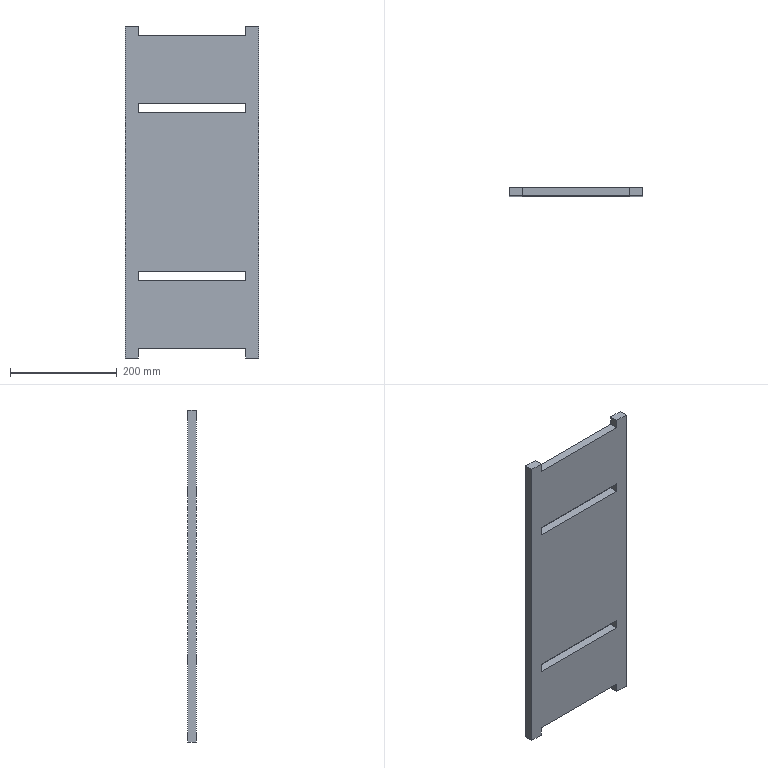Part | SolidWorks | features Extrusion 1 | 1 solid | 22 faces | box 250 x 16 x 623 mm | volume 2273312 mm3 | plane 22
STEP:
#1=CARTESIAN_POINT('',(-100.5,0.,165.5));
#2=VERTEX_POINT('',#1);
#3=CARTESIAN_POINT('',(100.5,0.,165.5));
#4=VERTEX_POINT('',#3);
#5=CARTESIAN_POINT('',(0.,0.,165.5));
#6=DIRECTION('',(1.,0.,0.));
#7=VECTOR('',#6,1000.);
#8=LINE('',#5,#7);
#9=EDGE_CURVE('',#2,#4,#8,.T.);
#10=ORIENTED_EDGE('',*,*,#9,.F.);
#11=CARTESIAN_POINT('',(-100.5,16.,165.5));
#12=VERTEX_POINT('',#11);
#13=CARTESIAN_POINT('',(-100.5,16.,165.5));
#14=DIRECTION('',(0.,-1.,0.));
#15=VECTOR('',#14,1000.);
#16=LINE('',#13,#15);
#17=EDGE_CURVE('',#12,#2,#16,.T.);
#18=ORIENTED_EDGE('',*,*,#17,.F.);
#19=CARTESIAN_POINT('',(100.5,16.,165.5));
#20=VERTEX_POINT('',#19);
#21=CARTESIAN_POINT('',(0.,16.,165.5));
#22=DIRECTION('',(1.,0.,0.));
#23=VECTOR('',#22,1000.);
#24=LINE('',#21,#23);
#25=EDGE_CURVE('',#12,#20,#24,.T.);
#26=ORIENTED_EDGE('',*,*,#25,.T.);
#27=CARTESIAN_POINT('',(100.5,16.,165.5));
#28=DIRECTION('',(0.,-1.,0.));
#29=VECTOR('',#28,1000.);
#30=LINE('',#27,#29);
#31=EDGE_CURVE('',#20,#4,#30,.T.);
#32=ORIENTED_EDGE('',*,*,#31,.T.);
#33=EDGE_LOOP('',(#10,#18,#26,#32));
#34=FACE_OUTER_BOUND('',#33,.T.);
#35=CARTESIAN_POINT('',(0.,16.,165.5));
#36=DIRECTION('',(0.,0.,-1.));
#37=DIRECTION('',(-1.,0.,0.));
#38=AXIS2_PLACEMENT_3D('',#35,#36,#37);
#39=PLANE('',#38);
#40=ADVANCED_FACE('',(#34),#39,.T.);
#41=CARTESIAN_POINT('',(-100.5,0.,148.5));
#42=VERTEX_POINT('',#41);
#43=CARTESIAN_POINT('',(-100.5,0.,0.));
#44=DIRECTION('',(0.,0.,-1.));
#45=VECTOR('',#44,1000.);
#46=LINE('',#43,#45);
#47=EDGE_CURVE('',#2,#42,#46,.T.);
#48=ORIENTED_EDGE('',*,*,#47,.T.);
#49=CARTESIAN_POINT('',(-100.5,16.,148.5));
#50=VERTEX_POINT('',#49);
#51=CARTESIAN_POINT('',(-100.5,16.,148.5));
#52=DIRECTION('',(0.,-1.,0.));
#53=VECTOR('',#52,1000.);
#54=LINE('',#51,#53);
#55=EDGE_CURVE('',#50,#42,#54,.T.);
#56=ORIENTED_EDGE('',*,*,#55,.F.);
#57=CARTESIAN_POINT('',(-100.5,16.,0.));
#58=DIRECTION('',(0.,0.,-1.));
#59=VECTOR('',#58,1000.);
#60=LINE('',#57,#59);
#61=EDGE_CURVE('',#12,#50,#60,.T.);
#62=ORIENTED_EDGE('',*,*,#61,.F.);
#63=ORIENTED_EDGE('',*,*,#17,.T.);
#64=EDGE_LOOP('',(#48,#56,#62,#63));
#65=FACE_OUTER_BOUND('',#64,.T.);
#66=CARTESIAN_POINT('',(-100.5,16.,0.));
#67=DIRECTION('',(-1.,0.,0.));
#68=DIRECTION('',(0.,0.,1.));
#69=AXIS2_PLACEMENT_3D('',#66,#67,#68);
#70=PLANE('',#69);
#71=ADVANCED_FACE('',(#65),#70,.F.);
#72=CARTESIAN_POINT('',(100.5,0.,148.5));
#73=VERTEX_POINT('',#72);
#74=CARTESIAN_POINT('',(0.,0.,148.5));
#75=DIRECTION('',(1.,0.,0.));
#76=VECTOR('',#75,1000.);
#77=LINE('',#74,#76);
#78=EDGE_CURVE('',#42,#73,#77,.T.);
#79=ORIENTED_EDGE('',*,*,#78,.T.);
#80=CARTESIAN_POINT('',(100.5,16.,148.5));
#81=VERTEX_POINT('',#80);
#82=CARTESIAN_POINT('',(100.5,16.,148.5));
#83=DIRECTION('',(0.,-1.,0.));
#84=VECTOR('',#83,1000.);
#85=LINE('',#82,#84);
#86=EDGE_CURVE('',#81,#73,#85,.T.);
#87=ORIENTED_EDGE('',*,*,#86,.F.);
#88=CARTESIAN_POINT('',(0.,16.,148.5));
#89=DIRECTION('',(1.,0.,0.));
#90=VECTOR('',#89,1000.);
#91=LINE('',#88,#90);
#92=EDGE_CURVE('',#50,#81,#91,.T.);
#93=ORIENTED_EDGE('',*,*,#92,.F.);
#94=ORIENTED_EDGE('',*,*,#55,.T.);
#95=EDGE_LOOP('',(#79,#87,#93,#94));
#96=FACE_OUTER_BOUND('',#95,.T.);
#97=CARTESIAN_POINT('',(0.,16.,148.5));
#98=DIRECTION('',(0.,0.,-1.));
#99=DIRECTION('',(-1.,0.,0.));
#100=AXIS2_PLACEMENT_3D('',#97,#98,#99);
#101=PLANE('',#100);
#102=ADVANCED_FACE('',(#96),#101,.F.);
#103=CARTESIAN_POINT('',(-100.5,0.,-165.5));
#104=VERTEX_POINT('',#103);
#105=CARTESIAN_POINT('',(100.5,0.,-165.5));
#106=VERTEX_POINT('',#105);
#107=CARTESIAN_POINT('',(0.,0.,-165.5));
#108=DIRECTION('',(1.,0.,0.));
#109=VECTOR('',#108,1000.);
#110=LINE('',#107,#109);
#111=EDGE_CURVE('',#104,#106,#110,.T.);
#112=ORIENTED_EDGE('',*,*,#111,.T.);
#113=CARTESIAN_POINT('',(100.5,16.,-165.5));
#114=VERTEX_POINT('',#113);
#115=CARTESIAN_POINT('',(100.5,16.,-165.5));
#116=DIRECTION('',(0.,-1.,0.));
#117=VECTOR('',#116,1000.);
#118=LINE('',#115,#117);
#119=EDGE_CURVE('',#114,#106,#118,.T.);
#120=ORIENTED_EDGE('',*,*,#119,.F.);
#121=CARTESIAN_POINT('',(-100.5,16.,-165.5));
#122=VERTEX_POINT('',#121);
#123=CARTESIAN_POINT('',(0.,16.,-165.5));
#124=DIRECTION('',(1.,0.,0.));
#125=VECTOR('',#124,1000.);
#126=LINE('',#123,#125);
#127=EDGE_CURVE('',#122,#114,#126,.T.);
#128=ORIENTED_EDGE('',*,*,#127,.F.);
#129=CARTESIAN_POINT('',(-100.5,16.,-165.5));
#130=DIRECTION('',(0.,-1.,0.));
#131=VECTOR('',#130,1000.);
#132=LINE('',#129,#131);
#133=EDGE_CURVE('',#122,#104,#132,.T.);
#134=ORIENTED_EDGE('',*,*,#133,.T.);
#135=EDGE_LOOP('',(#112,#120,#128,#134));
#136=FACE_OUTER_BOUND('',#135,.T.);
#137=CARTESIAN_POINT('',(0.,16.,-165.5));
#138=DIRECTION('',(0.,0.,-1.));
#139=DIRECTION('',(-1.,0.,0.));
#140=AXIS2_PLACEMENT_3D('',#137,#138,#139);
#141=PLANE('',#140);
#142=ADVANCED_FACE('',(#136),#141,.F.);
#143=CARTESIAN_POINT('',(100.5,0.,-148.5));
#144=VERTEX_POINT('',#143);
#145=CARTESIAN_POINT('',(100.5,0.,0.));
#146=DIRECTION('',(0.,0.,1.));
#147=VECTOR('',#146,1000.);
#148=LINE('',#145,#147);
#149=EDGE_CURVE('',#106,#144,#148,.T.);
#150=ORIENTED_EDGE('',*,*,#149,.T.);
#151=CARTESIAN_POINT('',(100.5,16.,-148.5));
#152=VERTEX_POINT('',#151);
#153=CARTESIAN_POINT('',(100.5,16.,-148.5));
#154=DIRECTION('',(0.,-1.,0.));
#155=VECTOR('',#154,1000.);
#156=LINE('',#153,#155);
#157=EDGE_CURVE('',#152,#144,#156,.T.);
#158=ORIENTED_EDGE('',*,*,#157,.F.);
#159=CARTESIAN_POINT('',(100.5,16.,0.));
#160=DIRECTION('',(0.,0.,1.));
#161=VECTOR('',#160,1000.);
#162=LINE('',#159,#161);
#163=EDGE_CURVE('',#114,#152,#162,.T.);
#164=ORIENTED_EDGE('',*,*,#163,.F.);
#165=ORIENTED_EDGE('',*,*,#119,.T.);
#166=EDGE_LOOP('',(#150,#158,#164,#165));
#167=FACE_OUTER_BOUND('',#166,.T.);
#168=CARTESIAN_POINT('',(100.5,16.,0.));
#169=DIRECTION('',(1.,0.,0.));
#170=DIRECTION('',(0.,0.,-1.));
#171=AXIS2_PLACEMENT_3D('',#168,#169,#170);
#172=PLANE('',#171);
#173=ADVANCED_FACE('',(#167),#172,.F.);
#174=CARTESIAN_POINT('',(-100.5,0.,-148.5));
#175=VERTEX_POINT('',#174);
#176=CARTESIAN_POINT('',(0.,0.,-148.5));
#177=DIRECTION('',(1.,0.,0.));
#178=VECTOR('',#177,1000.);
#179=LINE('',#176,#178);
#180=EDGE_CURVE('',#175,#144,#179,.T.);
#181=ORIENTED_EDGE('',*,*,#180,.F.);
#182=CARTESIAN_POINT('',(-100.5,16.,-148.5));
#183=VERTEX_POINT('',#182);
#184=CARTESIAN_POINT('',(-100.5,16.,-148.5));
#185=DIRECTION('',(0.,-1.,0.));
#186=VECTOR('',#185,1000.);
#187=LINE('',#184,#186);
#188=EDGE_CURVE('',#183,#175,#187,.T.);
#189=ORIENTED_EDGE('',*,*,#188,.F.);
#190=CARTESIAN_POINT('',(0.,16.,-148.5));
#191=DIRECTION('',(1.,0.,0.));
#192=VECTOR('',#191,1000.);
#193=LINE('',#190,#192);
#194=EDGE_CURVE('',#183,#152,#193,.T.);
#195=ORIENTED_EDGE('',*,*,#194,.T.);
#196=ORIENTED_EDGE('',*,*,#157,.T.);
#197=EDGE_LOOP('',(#181,#189,#195,#196));
#198=FACE_OUTER_BOUND('',#197,.T.);
#199=CARTESIAN_POINT('',(0.,16.,-148.5));
#200=DIRECTION('',(0.,0.,-1.));
#201=DIRECTION('',(-1.,0.,0.));
#202=AXIS2_PLACEMENT_3D('',#199,#200,#201);
#203=PLANE('',#202);
#204=ADVANCED_FACE('',(#198),#203,.T.);
#205=CARTESIAN_POINT('',(100.5,0.,311.5));
#206=VERTEX_POINT('',#205);
#207=CARTESIAN_POINT('',(100.5,0.,294.5));
#208=VERTEX_POINT('',#207);
#209=CARTESIAN_POINT('',(100.5,0.,0.));
#210=DIRECTION('',(0.,0.,-1.));
#211=VECTOR('',#210,1000.);
#212=LINE('',#209,#211);
#213=EDGE_CURVE('',#206,#208,#212,.T.);
#214=ORIENTED_EDGE('',*,*,#213,.F.);
#215=CARTESIAN_POINT('',(100.5,16.,311.5));
#216=VERTEX_POINT('',#215);
#217=CARTESIAN_POINT('',(100.5,16.,311.5));
#218=DIRECTION('',(0.,-1.,0.));
#219=VECTOR('',#218,1000.);
#220=LINE('',#217,#219);
#221=EDGE_CURVE('',#216,#206,#220,.T.);
#222=ORIENTED_EDGE('',*,*,#221,.F.);
#223=CARTESIAN_POINT('',(100.5,16.,294.5));
#224=VERTEX_POINT('',#223);
#225=CARTESIAN_POINT('',(100.5,16.,0.));
#226=DIRECTION('',(0.,0.,-1.));
#227=VECTOR('',#226,1000.);
#228=LINE('',#225,#227);
#229=EDGE_CURVE('',#216,#224,#228,.T.);
#230=ORIENTED_EDGE('',*,*,#229,.T.);
#231=CARTESIAN_POINT('',(100.5,16.,294.5));
#232=DIRECTION('',(0.,-1.,0.));
#233=VECTOR('',#232,1000.);
#234=LINE('',#231,#233);
#235=EDGE_CURVE('',#224,#208,#234,.T.);
#236=ORIENTED_EDGE('',*,*,#235,.T.);
#237=EDGE_LOOP('',(#214,#222,#230,#236));
#238=FACE_OUTER_BOUND('',#237,.T.);
#239=CARTESIAN_POINT('',(100.5,16.,0.));
#240=DIRECTION('',(-1.,0.,0.));
#241=DIRECTION('',(0.,0.,1.));
#242=AXIS2_PLACEMENT_3D('',#239,#240,#241);
#243=PLANE('',#242);
#244=ADVANCED_FACE('',(#238),#243,.T.);
#245=CARTESIAN_POINT('',(125.,0.,311.5));
#246=VERTEX_POINT('',#245);
#247=CARTESIAN_POINT('',(0.,0.,311.5));
#248=DIRECTION('',(1.,0.,0.));
#249=VECTOR('',#248,1000.);
#250=LINE('',#247,#249);
#251=EDGE_CURVE('',#206,#246,#250,.T.);
#252=ORIENTED_EDGE('',*,*,#251,.T.);
#253=CARTESIAN_POINT('',(125.,16.,311.5));
#254=VERTEX_POINT('',#253);
#255=CARTESIAN_POINT('',(125.,16.,311.5));
#256=DIRECTION('',(0.,-1.,0.));
#257=VECTOR('',#256,1000.);
#258=LINE('',#255,#257);
#259=EDGE_CURVE('',#254,#246,#258,.T.);
#260=ORIENTED_EDGE('',*,*,#259,.F.);
#261=CARTESIAN_POINT('',(0.,16.,311.5));
#262=DIRECTION('',(1.,0.,0.));
#263=VECTOR('',#262,1000.);
#264=LINE('',#261,#263);
#265=EDGE_CURVE('',#216,#254,#264,.T.);
#266=ORIENTED_EDGE('',*,*,#265,.F.);
#267=ORIENTED_EDGE('',*,*,#221,.T.);
#268=EDGE_LOOP('',(#252,#260,#266,#267));
#269=FACE_OUTER_BOUND('',#268,.T.);
#270=CARTESIAN_POINT('',(0.,16.,311.5));
#271=DIRECTION('',(0.,0.,-1.));
#272=DIRECTION('',(-1.,0.,0.));
#273=AXIS2_PLACEMENT_3D('',#270,#271,#272);
#274=PLANE('',#273);
#275=ADVANCED_FACE('',(#269),#274,.F.);
#276=CARTESIAN_POINT('',(125.,0.,-311.5));
#277=VERTEX_POINT('',#276);
#278=CARTESIAN_POINT('',(125.,0.,0.));
#279=DIRECTION('',(0.,0.,-1.));
#280=VECTOR('',#279,1000.);
#281=LINE('',#278,#280);
#282=EDGE_CURVE('',#246,#277,#281,.T.);
#283=ORIENTED_EDGE('',*,*,#282,.T.);
#284=CARTESIAN_POINT('',(125.,16.,-311.5));
#285=VERTEX_POINT('',#284);
#286=CARTESIAN_POINT('',(125.,16.,-311.5));
#287=DIRECTION('',(0.,-1.,0.));
#288=VECTOR('',#287,1000.);
#289=LINE('',#286,#288);
#290=EDGE_CURVE('',#285,#277,#289,.T.);
#291=ORIENTED_EDGE('',*,*,#290,.F.);
#292=CARTESIAN_POINT('',(125.,16.,0.));
#293=DIRECTION('',(0.,0.,-1.));
#294=VECTOR('',#293,1000.);
#295=LINE('',#292,#294);
#296=EDGE_CURVE('',#254,#285,#295,.T.);
#297=ORIENTED_EDGE('',*,*,#296,.F.);
#298=ORIENTED_EDGE('',*,*,#259,.T.);
#299=EDGE_LOOP('',(#283,#291,#297,#298));
#300=FACE_OUTER_BOUND('',#299,.T.);
#301=CARTESIAN_POINT('',(125.,16.,0.));
#302=DIRECTION('',(-1.,0.,0.));
#303=DIRECTION('',(0.,0.,1.));
#304=AXIS2_PLACEMENT_3D('',#301,#302,#303);
#305=PLANE('',#304);
#306=ADVANCED_FACE('',(#300),#305,.F.);
#307=CARTESIAN_POINT('',(100.5,0.,-311.5));
#308=VERTEX_POINT('',#307);
#309=CARTESIAN_POINT('',(0.,0.,-311.5));
#310=DIRECTION('',(1.,0.,0.));
#311=VECTOR('',#310,1000.);
#312=LINE('',#309,#311);
#313=EDGE_CURVE('',#308,#277,#312,.T.);
#314=ORIENTED_EDGE('',*,*,#313,.F.);
#315=CARTESIAN_POINT('',(100.5,16.,-311.5));
#316=VERTEX_POINT('',#315);
#317=CARTESIAN_POINT('',(100.5,16.,-311.5));
#318=DIRECTION('',(0.,-1.,0.));
#319=VECTOR('',#318,1000.);
#320=LINE('',#317,#319);
#321=EDGE_CURVE('',#316,#308,#320,.T.);
#322=ORIENTED_EDGE('',*,*,#321,.F.);
#323=CARTESIAN_POINT('',(0.,16.,-311.5));
#324=DIRECTION('',(1.,0.,0.));
#325=VECTOR('',#324,1000.);
#326=LINE('',#323,#325);
#327=EDGE_CURVE('',#316,#285,#326,.T.);
#328=ORIENTED_EDGE('',*,*,#327,.T.);
#329=ORIENTED_EDGE('',*,*,#290,.T.);
#330=EDGE_LOOP('',(#314,#322,#328,#329));
#331=FACE_OUTER_BOUND('',#330,.T.);
#332=CARTESIAN_POINT('',(0.,16.,-311.5));
#333=DIRECTION('',(0.,0.,-1.));
#334=DIRECTION('',(-1.,0.,0.));
#335=AXIS2_PLACEMENT_3D('',#332,#333,#334);
#336=PLANE('',#335);
#337=ADVANCED_FACE('',(#331),#336,.T.);
#338=CARTESIAN_POINT('',(100.5,0.,-294.5));
#339=VERTEX_POINT('',#338);
#340=CARTESIAN_POINT('',(100.5,0.,0.));
#341=DIRECTION('',(0.,0.,1.));
#342=VECTOR('',#341,1000.);
#343=LINE('',#340,#342);
#344=EDGE_CURVE('',#308,#339,#343,.T.);
#345=ORIENTED_EDGE('',*,*,#344,.T.);
#346=CARTESIAN_POINT('',(100.5,16.,-294.5));
#347=VERTEX_POINT('',#346);
#348=CARTESIAN_POINT('',(100.5,16.,-294.5));
#349=DIRECTION('',(0.,-1.,0.));
#350=VECTOR('',#349,1000.);
#351=LINE('',#348,#350);
#352=EDGE_CURVE('',#347,#339,#351,.T.);
#353=ORIENTED_EDGE('',*,*,#352,.F.);
#354=CARTESIAN_POINT('',(100.5,16.,0.));
#355=DIRECTION('',(0.,0.,1.));
#356=VECTOR('',#355,1000.);
#357=LINE('',#354,#356);
#358=EDGE_CURVE('',#316,#347,#357,.T.);
#359=ORIENTED_EDGE('',*,*,#358,.F.);
#360=ORIENTED_EDGE('',*,*,#321,.T.);
#361=EDGE_LOOP('',(#345,#353,#359,#360));
#362=FACE_OUTER_BOUND('',#361,.T.);
#363=CARTESIAN_POINT('',(100.5,16.,0.));
#364=DIRECTION('',(1.,0.,0.));
#365=DIRECTION('',(0.,0.,-1.));
#366=AXIS2_PLACEMENT_3D('',#363,#364,#365);
#367=PLANE('',#366);
#368=ADVANCED_FACE('',(#362),#367,.F.);
#369=CARTESIAN_POINT('',(-100.5,0.,-294.5));
#370=VERTEX_POINT('',#369);
#371=CARTESIAN_POINT('',(0.,0.,-294.5));
#372=DIRECTION('',(1.,0.,0.));
#373=VECTOR('',#372,1000.);
#374=LINE('',#371,#373);
#375=EDGE_CURVE('',#370,#339,#374,.T.);
#376=ORIENTED_EDGE('',*,*,#375,.F.);
#377=CARTESIAN_POINT('',(-100.5,16.,-294.5));
#378=VERTEX_POINT('',#377);
#379=CARTESIAN_POINT('',(-100.5,16.,-294.5));
#380=DIRECTION('',(0.,-1.,0.));
#381=VECTOR('',#380,1000.);
#382=LINE('',#379,#381);
#383=EDGE_CURVE('',#378,#370,#382,.T.);
#384=ORIENTED_EDGE('',*,*,#383,.F.);
#385=CARTESIAN_POINT('',(0.,16.,-294.5));
#386=DIRECTION('',(1.,0.,0.));
#387=VECTOR('',#386,1000.);
#388=LINE('',#385,#387);
#389=EDGE_CURVE('',#378,#347,#388,.T.);
#390=ORIENTED_EDGE('',*,*,#389,.T.);
#391=ORIENTED_EDGE('',*,*,#352,.T.);
#392=EDGE_LOOP('',(#376,#384,#390,#391));
#393=FACE_OUTER_BOUND('',#392,.T.);
#394=CARTESIAN_POINT('',(0.,16.,-294.5));
#395=DIRECTION('',(0.,0.,-1.));
#396=DIRECTION('',(-1.,0.,0.));
#397=AXIS2_PLACEMENT_3D('',#394,#395,#396);
#398=PLANE('',#397);
#399=ADVANCED_FACE('',(#393),#398,.T.);
#400=CARTESIAN_POINT('',(-100.5,0.,-311.5));
#401=VERTEX_POINT('',#400);
#402=CARTESIAN_POINT('',(-100.5,0.,0.));
#403=DIRECTION('',(0.,0.,1.));
#404=VECTOR('',#403,1000.);
#405=LINE('',#402,#404);
#406=EDGE_CURVE('',#401,#370,#405,.T.);
#407=ORIENTED_EDGE('',*,*,#406,.F.);
#408=CARTESIAN_POINT('',(-100.5,16.,-311.5));
#409=VERTEX_POINT('',#408);
#410=CARTESIAN_POINT('',(-100.5,16.,-311.5));
#411=DIRECTION('',(0.,-1.,0.));
#412=VECTOR('',#411,1000.);
#413=LINE('',#410,#412);
#414=EDGE_CURVE('',#409,#401,#413,.T.);
#415=ORIENTED_EDGE('',*,*,#414,.F.);
#416=CARTESIAN_POINT('',(-100.5,16.,0.));
#417=DIRECTION('',(0.,0.,1.));
#418=VECTOR('',#417,1000.);
#419=LINE('',#416,#418);
#420=EDGE_CURVE('',#409,#378,#419,.T.);
#421=ORIENTED_EDGE('',*,*,#420,.T.);
#422=ORIENTED_EDGE('',*,*,#383,.T.);
#423=EDGE_LOOP('',(#407,#415,#421,#422));
#424=FACE_OUTER_BOUND('',#423,.T.);
#425=CARTESIAN_POINT('',(-100.5,16.,0.));
#426=DIRECTION('',(1.,0.,0.));
#427=DIRECTION('',(0.,0.,-1.));
#428=AXIS2_PLACEMENT_3D('',#425,#426,#427);
#429=PLANE('',#428);
#430=ADVANCED_FACE('',(#424),#429,.T.);
#431=CARTESIAN_POINT('',(-125.,0.,-311.5));
#432=VERTEX_POINT('',#431);
#433=CARTESIAN_POINT('',(0.,0.,-311.5));
#434=DIRECTION('',(1.,0.,0.));
#435=VECTOR('',#434,1000.);
#436=LINE('',#433,#435);
#437=EDGE_CURVE('',#432,#401,#436,.T.);
#438=ORIENTED_EDGE('',*,*,#437,.F.);
#439=CARTESIAN_POINT('',(-125.,16.,-311.5));
#440=VERTEX_POINT('',#439);
#441=CARTESIAN_POINT('',(-125.,16.,-311.5));
#442=DIRECTION('',(0.,-1.,0.));
#443=VECTOR('',#442,1000.);
#444=LINE('',#441,#443);
#445=EDGE_CURVE('',#440,#432,#444,.T.);
#446=ORIENTED_EDGE('',*,*,#445,.F.);
#447=CARTESIAN_POINT('',(0.,16.,-311.5));
#448=DIRECTION('',(1.,0.,0.));
#449=VECTOR('',#448,1000.);
#450=LINE('',#447,#449);
#451=EDGE_CURVE('',#440,#409,#450,.T.);
#452=ORIENTED_EDGE('',*,*,#451,.T.);
#453=ORIENTED_EDGE('',*,*,#414,.T.);
#454=EDGE_LOOP('',(#438,#446,#452,#453));
#455=FACE_OUTER_BOUND('',#454,.T.);
#456=CARTESIAN_POINT('',(0.,16.,-311.5));
#457=DIRECTION('',(0.,0.,-1.));
#458=DIRECTION('',(-1.,0.,0.));
#459=AXIS2_PLACEMENT_3D('',#456,#457,#458);
#460=PLANE('',#459);
#461=ADVANCED_FACE('',(#455),#460,.T.);
#462=CARTESIAN_POINT('',(-125.,0.,311.5));
#463=VERTEX_POINT('',#462);
#464=CARTESIAN_POINT('',(-125.,0.,0.));
#465=DIRECTION('',(0.,0.,-1.));
#466=VECTOR('',#465,1000.);
#467=LINE('',#464,#466);
#468=EDGE_CURVE('',#463,#432,#467,.T.);
#469=ORIENTED_EDGE('',*,*,#468,.F.);
#470=CARTESIAN_POINT('',(-125.,16.,311.5));
#471=VERTEX_POINT('',#470);
#472=CARTESIAN_POINT('',(-125.,16.,311.5));
#473=DIRECTION('',(0.,-1.,0.));
#474=VECTOR('',#473,1000.);
#475=LINE('',#472,#474);
#476=EDGE_CURVE('',#471,#463,#475,.T.);
#477=ORIENTED_EDGE('',*,*,#476,.F.);
#478=CARTESIAN_POINT('',(-125.,16.,0.));
#479=DIRECTION('',(0.,0.,-1.));
#480=VECTOR('',#479,1000.);
#481=LINE('',#478,#480);
#482=EDGE_CURVE('',#471,#440,#481,.T.);
#483=ORIENTED_EDGE('',*,*,#482,.T.);
#484=ORIENTED_EDGE('',*,*,#445,.T.);
#485=EDGE_LOOP('',(#469,#477,#483,#484));
#486=FACE_OUTER_BOUND('',#485,.T.);
#487=CARTESIAN_POINT('',(-125.,16.,0.));
#488=DIRECTION('',(-1.,0.,0.));
#489=DIRECTION('',(0.,0.,1.));
#490=AXIS2_PLACEMENT_3D('',#487,#488,#489);
#491=PLANE('',#490);
#492=ADVANCED_FACE('',(#486),#491,.T.);
#493=CARTESIAN_POINT('',(-100.5,0.,311.5));
#494=VERTEX_POINT('',#493);
#495=CARTESIAN_POINT('',(0.,0.,311.5));
#496=DIRECTION('',(1.,0.,0.));
#497=VECTOR('',#496,1000.);
#498=LINE('',#495,#497);
#499=EDGE_CURVE('',#463,#494,#498,.T.);
#500=ORIENTED_EDGE('',*,*,#499,.T.);
#501=CARTESIAN_POINT('',(-100.5,16.,311.5));
#502=VERTEX_POINT('',#501);
#503=CARTESIAN_POINT('',(-100.5,16.,311.5));
#504=DIRECTION('',(0.,-1.,0.));
#505=VECTOR('',#504,1000.);
#506=LINE('',#503,#505);
#507=EDGE_CURVE('',#502,#494,#506,.T.);
#508=ORIENTED_EDGE('',*,*,#507,.F.);
#509=CARTESIAN_POINT('',(0.,16.,311.5));
#510=DIRECTION('',(1.,0.,0.));
#511=VECTOR('',#510,1000.);
#512=LINE('',#509,#511);
#513=EDGE_CURVE('',#471,#502,#512,.T.);
#514=ORIENTED_EDGE('',*,*,#513,.F.);
#515=ORIENTED_EDGE('',*,*,#476,.T.);
#516=EDGE_LOOP('',(#500,#508,#514,#515));
#517=FACE_OUTER_BOUND('',#516,.T.);
#518=CARTESIAN_POINT('',(0.,16.,311.5));
#519=DIRECTION('',(0.,0.,-1.));
#520=DIRECTION('',(-1.,0.,0.));
#521=AXIS2_PLACEMENT_3D('',#518,#519,#520);
#522=PLANE('',#521);
#523=ADVANCED_FACE('',(#517),#522,.F.);
#524=CARTESIAN_POINT('',(-100.5,0.,294.5));
#525=VERTEX_POINT('',#524);
#526=CARTESIAN_POINT('',(-100.5,0.,0.));
#527=DIRECTION('',(0.,0.,-1.));
#528=VECTOR('',#527,1000.);
#529=LINE('',#526,#528);
#530=EDGE_CURVE('',#494,#525,#529,.T.);
#531=ORIENTED_EDGE('',*,*,#530,.T.);
#532=CARTESIAN_POINT('',(-100.5,16.,294.5));
#533=VERTEX_POINT('',#532);
#534=CARTESIAN_POINT('',(-100.5,16.,294.5));
#535=DIRECTION('',(0.,-1.,0.));
#536=VECTOR('',#535,1000.);
#537=LINE('',#534,#536);
#538=EDGE_CURVE('',#533,#525,#537,.T.);
#539=ORIENTED_EDGE('',*,*,#538,.F.);
#540=CARTESIAN_POINT('',(-100.5,16.,0.));
#541=DIRECTION('',(0.,0.,-1.));
#542=VECTOR('',#541,1000.);
#543=LINE('',#540,#542);
#544=EDGE_CURVE('',#502,#533,#543,.T.);
#545=ORIENTED_EDGE('',*,*,#544,.F.);
#546=ORIENTED_EDGE('',*,*,#507,.T.);
#547=EDGE_LOOP('',(#531,#539,#545,#546));
#548=FACE_OUTER_BOUND('',#547,.T.);
#549=CARTESIAN_POINT('',(-100.5,16.,0.));
#550=DIRECTION('',(-1.,0.,0.));
#551=DIRECTION('',(0.,0.,1.));
#552=AXIS2_PLACEMENT_3D('',#549,#550,#551);
#553=PLANE('',#552);
#554=ADVANCED_FACE('',(#548),#553,.F.);
#555=CARTESIAN_POINT('',(-100.5,0.,0.));
#556=DIRECTION('',(0.,0.,1.));
#557=VECTOR('',#556,1000.);
#558=LINE('',#555,#557);
#559=EDGE_CURVE('',#104,#175,#558,.T.);
#560=ORIENTED_EDGE('',*,*,#559,.F.);
#561=ORIENTED_EDGE('',*,*,#133,.F.);
#562=CARTESIAN_POINT('',(-100.5,16.,0.));
#563=DIRECTION('',(0.,0.,1.));
#564=VECTOR('',#563,1000.);
#565=LINE('',#562,#564);
#566=EDGE_CURVE('',#122,#183,#565,.T.);
#567=ORIENTED_EDGE('',*,*,#566,.T.);
#568=ORIENTED_EDGE('',*,*,#188,.T.);
#569=EDGE_LOOP('',(#560,#561,#567,#568));
#570=FACE_OUTER_BOUND('',#569,.T.);
#571=CARTESIAN_POINT('',(-100.5,16.,0.));
#572=DIRECTION('',(1.,0.,0.));
#573=DIRECTION('',(0.,0.,-1.));
#574=AXIS2_PLACEMENT_3D('',#571,#572,#573);
#575=PLANE('',#574);
#576=ADVANCED_FACE('',(#570),#575,.T.);
#577=CARTESIAN_POINT('',(0.,0.,294.5));
#578=DIRECTION('',(1.,0.,0.));
#579=VECTOR('',#578,1000.);
#580=LINE('',#577,#579);
#581=EDGE_CURVE('',#525,#208,#580,.T.);
#582=ORIENTED_EDGE('',*,*,#581,.T.);
#583=ORIENTED_EDGE('',*,*,#235,.F.);
#584=CARTESIAN_POINT('',(0.,16.,294.5));
#585=DIRECTION('',(1.,0.,0.));
#586=VECTOR('',#585,1000.);
#587=LINE('',#584,#586);
#588=EDGE_CURVE('',#533,#224,#587,.T.);
#589=ORIENTED_EDGE('',*,*,#588,.F.);
#590=ORIENTED_EDGE('',*,*,#538,.T.);
#591=EDGE_LOOP('',(#582,#583,#589,#590));
#592=FACE_OUTER_BOUND('',#591,.T.);
#593=CARTESIAN_POINT('',(0.,16.,294.5));
#594=DIRECTION('',(0.,0.,-1.));
#595=DIRECTION('',(-1.,0.,0.));
#596=AXIS2_PLACEMENT_3D('',#593,#594,#595);
#597=PLANE('',#596);
#598=ADVANCED_FACE('',(#592),#597,.F.);
#599=CARTESIAN_POINT('',(100.5,0.,0.));
#600=DIRECTION('',(0.,0.,-1.));
#601=VECTOR('',#600,1000.);
#602=LINE('',#599,#601);
#603=EDGE_CURVE('',#4,#73,#602,.T.);
#604=ORIENTED_EDGE('',*,*,#603,.F.);
#605=ORIENTED_EDGE('',*,*,#31,.F.);
#606=CARTESIAN_POINT('',(100.5,16.,0.));
#607=DIRECTION('',(0.,0.,-1.));
#608=VECTOR('',#607,1000.);
#609=LINE('',#606,#608);
#610=EDGE_CURVE('',#20,#81,#609,.T.);
#611=ORIENTED_EDGE('',*,*,#610,.T.);
#612=ORIENTED_EDGE('',*,*,#86,.T.);
#613=EDGE_LOOP('',(#604,#605,#611,#612));
#614=FACE_OUTER_BOUND('',#613,.T.);
#615=CARTESIAN_POINT('',(100.5,16.,0.));
#616=DIRECTION('',(-1.,0.,0.));
#617=DIRECTION('',(0.,0.,1.));
#618=AXIS2_PLACEMENT_3D('',#615,#616,#617);
#619=PLANE('',#618);
#620=ADVANCED_FACE('',(#614),#619,.T.);
#621=ORIENTED_EDGE('',*,*,#229,.F.);
#622=ORIENTED_EDGE('',*,*,#265,.T.);
#623=ORIENTED_EDGE('',*,*,#296,.T.);
#624=ORIENTED_EDGE('',*,*,#327,.F.);
#625=ORIENTED_EDGE('',*,*,#358,.T.);
#626=ORIENTED_EDGE('',*,*,#389,.F.);
#627=ORIENTED_EDGE('',*,*,#420,.F.);
#628=ORIENTED_EDGE('',*,*,#451,.F.);
#629=ORIENTED_EDGE('',*,*,#482,.F.);
#630=ORIENTED_EDGE('',*,*,#513,.T.);
#631=ORIENTED_EDGE('',*,*,#544,.T.);
#632=ORIENTED_EDGE('',*,*,#588,.T.);
#633=EDGE_LOOP('',(#621,#622,#623,#624,#625,#626,#627,#628,#629,#630,#631,#632));
#634=FACE_OUTER_BOUND('',#633,.T.);
#635=ORIENTED_EDGE('',*,*,#127,.T.);
#636=ORIENTED_EDGE('',*,*,#163,.T.);
#637=ORIENTED_EDGE('',*,*,#194,.F.);
#638=ORIENTED_EDGE('',*,*,#566,.F.);
#639=EDGE_LOOP('',(#635,#636,#637,#638));
#640=FACE_BOUND('',#639,.T.);
#641=ORIENTED_EDGE('',*,*,#25,.F.);
#642=ORIENTED_EDGE('',*,*,#61,.T.);
#643=ORIENTED_EDGE('',*,*,#92,.T.);
#644=ORIENTED_EDGE('',*,*,#610,.F.);
#645=EDGE_LOOP('',(#641,#642,#643,#644));
#646=FACE_BOUND('',#645,.T.);
#647=CARTESIAN_POINT('',(0.,16.,0.));
#648=DIRECTION('',(0.,1.,0.));
#649=DIRECTION('',(0.,0.,1.));
#650=AXIS2_PLACEMENT_3D('',#647,#648,#649);
#651=PLANE('',#650);
#652=ADVANCED_FACE('',(#634,#640,#646),#651,.T.);
#653=ORIENTED_EDGE('',*,*,#213,.T.);
#654=ORIENTED_EDGE('',*,*,#581,.F.);
#655=ORIENTED_EDGE('',*,*,#530,.F.);
#656=ORIENTED_EDGE('',*,*,#499,.F.);
#657=ORIENTED_EDGE('',*,*,#468,.T.);
#658=ORIENTED_EDGE('',*,*,#437,.T.);
#659=ORIENTED_EDGE('',*,*,#406,.T.);
#660=ORIENTED_EDGE('',*,*,#375,.T.);
#661=ORIENTED_EDGE('',*,*,#344,.F.);
#662=ORIENTED_EDGE('',*,*,#313,.T.);
#663=ORIENTED_EDGE('',*,*,#282,.F.);
#664=ORIENTED_EDGE('',*,*,#251,.F.);
#665=EDGE_LOOP('',(#653,#654,#655,#656,#657,#658,#659,#660,#661,#662,#663,#664));
#666=FACE_OUTER_BOUND('',#665,.T.);
#667=ORIENTED_EDGE('',*,*,#111,.F.);
#668=ORIENTED_EDGE('',*,*,#559,.T.);
#669=ORIENTED_EDGE('',*,*,#180,.T.);
#670=ORIENTED_EDGE('',*,*,#149,.F.);
#671=EDGE_LOOP('',(#667,#668,#669,#670));
#672=FACE_BOUND('',#671,.T.);
#673=ORIENTED_EDGE('',*,*,#9,.T.);
#674=ORIENTED_EDGE('',*,*,#603,.T.);
#675=ORIENTED_EDGE('',*,*,#78,.F.);
#676=ORIENTED_EDGE('',*,*,#47,.F.);
#677=EDGE_LOOP('',(#673,#674,#675,#676));
#678=FACE_BOUND('',#677,.T.);
#679=CARTESIAN_POINT('',(0.,0.,0.));
#680=DIRECTION('',(0.,1.,0.));
#681=DIRECTION('',(0.,0.,1.));
#682=AXIS2_PLACEMENT_3D('',#679,#680,#681);
#683=PLANE('',#682);
#684=ADVANCED_FACE('',(#666,#672,#678),#683,.F.);
#685=CLOSED_SHELL('',(#40,#71,#102,#142,#173,#204,#244,#275,#306,#337,#368,#399,#430,#461,#492,#523,#554,#576,#598,#620,#652,#684));
#686=MANIFOLD_SOLID_BREP('',#685);
#687=CARTESIAN_POINT('',(0.,0.,0.));
#688=DIRECTION('',(0.,0.,1.));
#689=DIRECTION('',(1.,0.,0.));
#690=AXIS2_PLACEMENT_3D('',#687,#688,#689);
#691=(LENGTH_UNIT()NAMED_UNIT(*)SI_UNIT(.MILLI.,.METRE.));
#692=UNCERTAINTY_MEASURE_WITH_UNIT(LENGTH_MEASURE(0.00001),#691,'','');
#693=(NAMED_UNIT(*)PLANE_ANGLE_UNIT()SI_UNIT($,.RADIAN.));
#694=(NAMED_UNIT(*)SI_UNIT($,.STERADIAN.)SOLID_ANGLE_UNIT());
#695=(GEOMETRIC_REPRESENTATION_CONTEXT(3)GLOBAL_UNCERTAINTY_ASSIGNED_CONTEXT((#692))GLOBAL_UNIT_ASSIGNED_CONTEXT((#691,#693,#694))REPRESENTATION_CONTEXT('',''));
#696=ADVANCED_BREP_SHAPE_REPRESENTATION('',(#686,#690),#695);